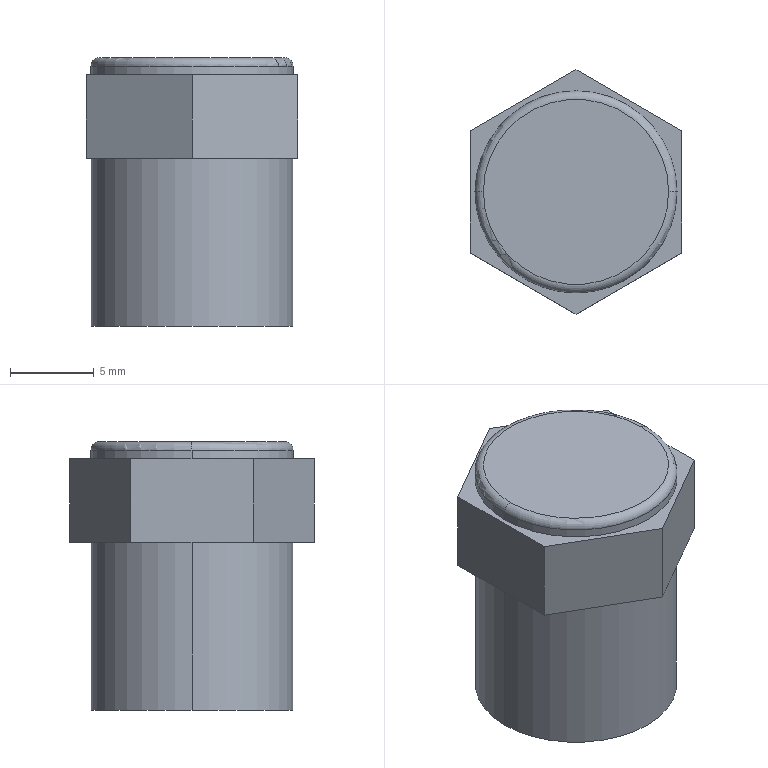Part | SolidWorks | features ICE 2, Extrusion 1, Fillet 1 | 1 solid | 16 faces | box 12.619 x 14.572 x 16 mm | volume 1932 mm3 | plane 10 | cylinder 4 | torus 2 | commonest cylinder face diameters 12 x2 12.036 x2
STEP:
#1=CARTESIAN_POINT('',(-6.018,0.,15.5));
#2=VERTEX_POINT('',#1);
#3=CARTESIAN_POINT('',(6.018,0.,15.5));
#4=VERTEX_POINT('',#3);
#5=CARTESIAN_POINT('',(0.,0.,15.5));
#6=DIRECTION('',(0.,0.,-1.));
#7=DIRECTION('',(1.,0.,0.));
#8=AXIS2_PLACEMENT_3D('',#5,#6,#7);
#9=CIRCLE('',#8,6.018);
#10=EDGE_CURVE('',#2,#4,#9,.T.);
#11=ORIENTED_EDGE('',*,*,#10,.F.);
#12=CARTESIAN_POINT('',(-5.518,0.,16.));
#13=VERTEX_POINT('',#12);
#14=CARTESIAN_POINT('',(-5.518,0.,15.5));
#15=DIRECTION('',(0.,1.,0.));
#16=DIRECTION('',(-1.,0.,0.));
#17=AXIS2_PLACEMENT_3D('',#14,#15,#16);
#18=CIRCLE('',#17,0.5);
#19=EDGE_CURVE('',#2,#13,#18,.T.);
#20=ORIENTED_EDGE('',*,*,#19,.T.);
#21=CARTESIAN_POINT('',(5.518,0.,16.));
#22=VERTEX_POINT('',#21);
#23=CARTESIAN_POINT('',(0.,0.,16.));
#24=DIRECTION('',(0.,0.,1.));
#25=DIRECTION('',(1.,0.,0.));
#26=AXIS2_PLACEMENT_3D('',#23,#24,#25);
#27=CIRCLE('',#26,5.518);
#28=EDGE_CURVE('',#22,#13,#27,.T.);
#29=ORIENTED_EDGE('',*,*,#28,.F.);
#30=CARTESIAN_POINT('',(5.518,0.,15.5));
#31=DIRECTION('',(0.,-1.,0.));
#32=DIRECTION('',(0.,0.,-1.));
#33=AXIS2_PLACEMENT_3D('',#30,#31,#32);
#34=CIRCLE('',#33,0.5);
#35=EDGE_CURVE('',#4,#22,#34,.T.);
#36=ORIENTED_EDGE('',*,*,#35,.F.);
#37=EDGE_LOOP('',(#11,#20,#29,#36));
#38=FACE_OUTER_BOUND('',#37,.T.);
#39=CARTESIAN_POINT('',(0.,0.,15.5));
#40=DIRECTION('',(0.,0.,1.));
#41=DIRECTION('',(1.,0.,0.));
#42=AXIS2_PLACEMENT_3D('',#39,#40,#41);
#43=TOROIDAL_SURFACE('',#42,5.518,0.5);
#44=ADVANCED_FACE('',(#38),#43,.T.);
#45=ORIENTED_EDGE('',*,*,#10,.T.);
#46=CARTESIAN_POINT('',(6.018,0.,15.));
#47=VERTEX_POINT('',#46);
#48=CARTESIAN_POINT('',(6.018,0.,16.));
#49=DIRECTION('',(0.,0.,-1.));
#50=VECTOR('',#49,1000.);
#51=LINE('',#48,#50);
#52=EDGE_CURVE('',#4,#47,#51,.T.);
#53=ORIENTED_EDGE('',*,*,#52,.T.);
#54=CARTESIAN_POINT('',(-6.018,0.,15.));
#55=VERTEX_POINT('',#54);
#56=CARTESIAN_POINT('',(0.,0.,15.));
#57=DIRECTION('',(0.,0.,1.));
#58=DIRECTION('',(1.,0.,0.));
#59=AXIS2_PLACEMENT_3D('',#56,#57,#58);
#60=CIRCLE('',#59,6.018);
#61=EDGE_CURVE('',#47,#55,#60,.T.);
#62=ORIENTED_EDGE('',*,*,#61,.T.);
#63=CARTESIAN_POINT('',(-6.018,0.,16.));
#64=DIRECTION('',(0.,0.,-1.));
#65=VECTOR('',#64,1000.);
#66=LINE('',#63,#65);
#67=EDGE_CURVE('',#2,#55,#66,.T.);
#68=ORIENTED_EDGE('',*,*,#67,.F.);
#69=EDGE_LOOP('',(#45,#53,#62,#68));
#70=FACE_OUTER_BOUND('',#69,.T.);
#71=CARTESIAN_POINT('',(0.,0.,16.));
#72=DIRECTION('',(0.,0.,-1.));
#73=DIRECTION('',(-1.,0.,0.));
#74=AXIS2_PLACEMENT_3D('',#71,#72,#73);
#75=CYLINDRICAL_SURFACE('',#74,6.018);
#76=ADVANCED_FACE('',(#70),#75,.T.);
#77=CARTESIAN_POINT('',(6.,0.,10.));
#78=VERTEX_POINT('',#77);
#79=CARTESIAN_POINT('',(-6.,0.,10.));
#80=VERTEX_POINT('',#79);
#81=CARTESIAN_POINT('',(0.,0.,10.));
#82=DIRECTION('',(0.,0.,1.));
#83=DIRECTION('',(1.,0.,0.));
#84=AXIS2_PLACEMENT_3D('',#81,#82,#83);
#85=CIRCLE('',#84,6.);
#86=EDGE_CURVE('',#78,#80,#85,.T.);
#87=ORIENTED_EDGE('',*,*,#86,.F.);
#88=CARTESIAN_POINT('',(6.,0.,0.));
#89=VERTEX_POINT('',#88);
#90=CARTESIAN_POINT('',(6.,0.,10.));
#91=DIRECTION('',(0.,0.,-1.));
#92=VECTOR('',#91,1000.);
#93=LINE('',#90,#92);
#94=EDGE_CURVE('',#78,#89,#93,.T.);
#95=ORIENTED_EDGE('',*,*,#94,.T.);
#96=CARTESIAN_POINT('',(-6.,0.,0.));
#97=VERTEX_POINT('',#96);
#98=CARTESIAN_POINT('',(0.,0.,0.));
#99=DIRECTION('',(0.,0.,1.));
#100=DIRECTION('',(1.,0.,0.));
#101=AXIS2_PLACEMENT_3D('',#98,#99,#100);
#102=CIRCLE('',#101,6.);
#103=EDGE_CURVE('',#89,#97,#102,.T.);
#104=ORIENTED_EDGE('',*,*,#103,.T.);
#105=CARTESIAN_POINT('',(-6.,0.,10.));
#106=DIRECTION('',(0.,0.,-1.));
#107=VECTOR('',#106,1000.);
#108=LINE('',#105,#107);
#109=EDGE_CURVE('',#80,#97,#108,.T.);
#110=ORIENTED_EDGE('',*,*,#109,.F.);
#111=EDGE_LOOP('',(#87,#95,#104,#110));
#112=FACE_OUTER_BOUND('',#111,.T.);
#113=CARTESIAN_POINT('',(0.,0.,10.));
#114=DIRECTION('',(0.,0.,-1.));
#115=DIRECTION('',(-1.,0.,0.));
#116=AXIS2_PLACEMENT_3D('',#113,#114,#115);
#117=CYLINDRICAL_SURFACE('',#116,6.);
#118=ADVANCED_FACE('',(#112),#117,.T.);
#119=ORIENTED_EDGE('',*,*,#94,.F.);
#120=CARTESIAN_POINT('',(0.,0.,10.));
#121=DIRECTION('',(0.,0.,1.));
#122=DIRECTION('',(1.,0.,0.));
#123=AXIS2_PLACEMENT_3D('',#120,#121,#122);
#124=CIRCLE('',#123,6.);
#125=EDGE_CURVE('',#80,#78,#124,.T.);
#126=ORIENTED_EDGE('',*,*,#125,.F.);
#127=ORIENTED_EDGE('',*,*,#109,.T.);
#128=CARTESIAN_POINT('',(0.,0.,0.));
#129=DIRECTION('',(0.,0.,1.));
#130=DIRECTION('',(1.,0.,0.));
#131=AXIS2_PLACEMENT_3D('',#128,#129,#130);
#132=CIRCLE('',#131,6.);
#133=EDGE_CURVE('',#97,#89,#132,.T.);
#134=ORIENTED_EDGE('',*,*,#133,.T.);
#135=EDGE_LOOP('',(#119,#126,#127,#134));
#136=FACE_OUTER_BOUND('',#135,.T.);
#137=CARTESIAN_POINT('',(0.,0.,10.));
#138=DIRECTION('',(0.,0.,-1.));
#139=DIRECTION('',(-1.,0.,0.));
#140=AXIS2_PLACEMENT_3D('',#137,#138,#139);
#141=CYLINDRICAL_SURFACE('',#140,6.);
#142=ADVANCED_FACE('',(#136),#141,.T.);
#143=ORIENTED_EDGE('',*,*,#133,.F.);
#144=ORIENTED_EDGE('',*,*,#103,.F.);
#145=EDGE_LOOP('',(#143,#144));
#146=FACE_OUTER_BOUND('',#145,.T.);
#147=CARTESIAN_POINT('',(0.,0.,0.));
#148=DIRECTION('',(0.,0.,1.));
#149=DIRECTION('',(1.,0.,0.));
#150=AXIS2_PLACEMENT_3D('',#147,#148,#149);
#151=PLANE('',#150);
#152=ADVANCED_FACE('',(#146),#151,.F.);
#153=CARTESIAN_POINT('',(6.31,3.643,10.));
#154=VERTEX_POINT('',#153);
#155=CARTESIAN_POINT('',(0.,7.286,10.));
#156=VERTEX_POINT('',#155);
#157=CARTESIAN_POINT('',(6.31,3.643,10.));
#158=DIRECTION('',(-0.866,0.5,0.));
#159=VECTOR('',#158,1000.);
#160=LINE('',#157,#159);
#161=EDGE_CURVE('',#154,#156,#160,.T.);
#162=ORIENTED_EDGE('',*,*,#161,.T.);
#163=CARTESIAN_POINT('',(0.,7.286,15.));
#164=VERTEX_POINT('',#163);
#165=CARTESIAN_POINT('',(0.,7.286,15.));
#166=DIRECTION('',(0.,0.,-1.));
#167=VECTOR('',#166,1000.);
#168=LINE('',#165,#167);
#169=EDGE_CURVE('',#164,#156,#168,.T.);
#170=ORIENTED_EDGE('',*,*,#169,.F.);
#171=CARTESIAN_POINT('',(6.31,3.643,15.));
#172=VERTEX_POINT('',#171);
#173=CARTESIAN_POINT('',(6.31,3.643,15.));
#174=DIRECTION('',(-0.866,0.5,0.));
#175=VECTOR('',#174,1000.);
#176=LINE('',#173,#175);
#177=EDGE_CURVE('',#172,#164,#176,.T.);
#178=ORIENTED_EDGE('',*,*,#177,.F.);
#179=CARTESIAN_POINT('',(6.31,3.643,15.));
#180=DIRECTION('',(0.,0.,-1.));
#181=VECTOR('',#180,1000.);
#182=LINE('',#179,#181);
#183=EDGE_CURVE('',#172,#154,#182,.T.);
#184=ORIENTED_EDGE('',*,*,#183,.T.);
#185=EDGE_LOOP('',(#162,#170,#178,#184));
#186=FACE_OUTER_BOUND('',#185,.T.);
#187=CARTESIAN_POINT('',(6.31,3.643,15.));
#188=DIRECTION('',(-0.5,-0.866,0.));
#189=DIRECTION('',(0.866,-0.5,0.));
#190=AXIS2_PLACEMENT_3D('',#187,#188,#189);
#191=PLANE('',#190);
#192=ADVANCED_FACE('',(#186),#191,.F.);
#193=CARTESIAN_POINT('',(-6.31,3.643,10.));
#194=VERTEX_POINT('',#193);
#195=CARTESIAN_POINT('',(0.,7.286,10.));
#196=DIRECTION('',(-0.866,-0.5,0.));
#197=VECTOR('',#196,1000.);
#198=LINE('',#195,#197);
#199=EDGE_CURVE('',#156,#194,#198,.T.);
#200=ORIENTED_EDGE('',*,*,#199,.T.);
#201=CARTESIAN_POINT('',(-6.31,3.643,15.));
#202=VERTEX_POINT('',#201);
#203=CARTESIAN_POINT('',(-6.31,3.643,15.));
#204=DIRECTION('',(0.,0.,-1.));
#205=VECTOR('',#204,1000.);
#206=LINE('',#203,#205);
#207=EDGE_CURVE('',#202,#194,#206,.T.);
#208=ORIENTED_EDGE('',*,*,#207,.F.);
#209=CARTESIAN_POINT('',(0.,7.286,15.));
#210=DIRECTION('',(-0.866,-0.5,0.));
#211=VECTOR('',#210,1000.);
#212=LINE('',#209,#211);
#213=EDGE_CURVE('',#164,#202,#212,.T.);
#214=ORIENTED_EDGE('',*,*,#213,.F.);
#215=ORIENTED_EDGE('',*,*,#169,.T.);
#216=EDGE_LOOP('',(#200,#208,#214,#215));
#217=FACE_OUTER_BOUND('',#216,.T.);
#218=CARTESIAN_POINT('',(0.,7.286,15.));
#219=DIRECTION('',(0.5,-0.866,0.));
#220=DIRECTION('',(0.866,0.5,0.));
#221=AXIS2_PLACEMENT_3D('',#218,#219,#220);
#222=PLANE('',#221);
#223=ADVANCED_FACE('',(#217),#222,.F.);
#224=CARTESIAN_POINT('',(-6.31,-3.643,10.));
#225=VERTEX_POINT('',#224);
#226=CARTESIAN_POINT('',(-6.31,3.643,10.));
#227=DIRECTION('',(0.,-1.,0.));
#228=VECTOR('',#227,1000.);
#229=LINE('',#226,#228);
#230=EDGE_CURVE('',#194,#225,#229,.T.);
#231=ORIENTED_EDGE('',*,*,#230,.T.);
#232=CARTESIAN_POINT('',(-6.31,-3.643,15.));
#233=VERTEX_POINT('',#232);
#234=CARTESIAN_POINT('',(-6.31,-3.643,15.));
#235=DIRECTION('',(0.,0.,-1.));
#236=VECTOR('',#235,1000.);
#237=LINE('',#234,#236);
#238=EDGE_CURVE('',#233,#225,#237,.T.);
#239=ORIENTED_EDGE('',*,*,#238,.F.);
#240=CARTESIAN_POINT('',(-6.31,3.643,15.));
#241=DIRECTION('',(0.,-1.,0.));
#242=VECTOR('',#241,1000.);
#243=LINE('',#240,#242);
#244=EDGE_CURVE('',#202,#233,#243,.T.);
#245=ORIENTED_EDGE('',*,*,#244,.F.);
#246=ORIENTED_EDGE('',*,*,#207,.T.);
#247=EDGE_LOOP('',(#231,#239,#245,#246));
#248=FACE_OUTER_BOUND('',#247,.T.);
#249=CARTESIAN_POINT('',(-6.31,3.643,15.));
#250=DIRECTION('',(1.,0.,0.));
#251=DIRECTION('',(0.,1.,0.));
#252=AXIS2_PLACEMENT_3D('',#249,#250,#251);
#253=PLANE('',#252);
#254=ADVANCED_FACE('',(#248),#253,.F.);
#255=CARTESIAN_POINT('',(0.,-7.286,10.));
#256=VERTEX_POINT('',#255);
#257=CARTESIAN_POINT('',(-6.31,-3.643,10.));
#258=DIRECTION('',(0.866,-0.5,0.));
#259=VECTOR('',#258,1000.);
#260=LINE('',#257,#259);
#261=EDGE_CURVE('',#225,#256,#260,.T.);
#262=ORIENTED_EDGE('',*,*,#261,.T.);
#263=CARTESIAN_POINT('',(0.,-7.286,15.));
#264=VERTEX_POINT('',#263);
#265=CARTESIAN_POINT('',(0.,-7.286,15.));
#266=DIRECTION('',(0.,0.,-1.));
#267=VECTOR('',#266,1000.);
#268=LINE('',#265,#267);
#269=EDGE_CURVE('',#264,#256,#268,.T.);
#270=ORIENTED_EDGE('',*,*,#269,.F.);
#271=CARTESIAN_POINT('',(-6.31,-3.643,15.));
#272=DIRECTION('',(0.866,-0.5,0.));
#273=VECTOR('',#272,1000.);
#274=LINE('',#271,#273);
#275=EDGE_CURVE('',#233,#264,#274,.T.);
#276=ORIENTED_EDGE('',*,*,#275,.F.);
#277=ORIENTED_EDGE('',*,*,#238,.T.);
#278=EDGE_LOOP('',(#262,#270,#276,#277));
#279=FACE_OUTER_BOUND('',#278,.T.);
#280=CARTESIAN_POINT('',(-6.31,-3.643,15.));
#281=DIRECTION('',(0.5,0.866,0.));
#282=DIRECTION('',(-0.866,0.5,0.));
#283=AXIS2_PLACEMENT_3D('',#280,#281,#282);
#284=PLANE('',#283);
#285=ADVANCED_FACE('',(#279),#284,.F.);
#286=CARTESIAN_POINT('',(6.31,-3.643,10.));
#287=VERTEX_POINT('',#286);
#288=CARTESIAN_POINT('',(0.,-7.286,10.));
#289=DIRECTION('',(0.866,0.5,0.));
#290=VECTOR('',#289,1000.);
#291=LINE('',#288,#290);
#292=EDGE_CURVE('',#256,#287,#291,.T.);
#293=ORIENTED_EDGE('',*,*,#292,.T.);
#294=CARTESIAN_POINT('',(6.31,-3.643,15.));
#295=VERTEX_POINT('',#294);
#296=CARTESIAN_POINT('',(6.31,-3.643,15.));
#297=DIRECTION('',(0.,0.,-1.));
#298=VECTOR('',#297,1000.);
#299=LINE('',#296,#298);
#300=EDGE_CURVE('',#295,#287,#299,.T.);
#301=ORIENTED_EDGE('',*,*,#300,.F.);
#302=CARTESIAN_POINT('',(0.,-7.286,15.));
#303=DIRECTION('',(0.866,0.5,0.));
#304=VECTOR('',#303,1000.);
#305=LINE('',#302,#304);
#306=EDGE_CURVE('',#264,#295,#305,.T.);
#307=ORIENTED_EDGE('',*,*,#306,.F.);
#308=ORIENTED_EDGE('',*,*,#269,.T.);
#309=EDGE_LOOP('',(#293,#301,#307,#308));
#310=FACE_OUTER_BOUND('',#309,.T.);
#311=CARTESIAN_POINT('',(0.,-7.286,15.));
#312=DIRECTION('',(-0.5,0.866,0.));
#313=DIRECTION('',(-0.866,-0.5,0.));
#314=AXIS2_PLACEMENT_3D('',#311,#312,#313);
#315=PLANE('',#314);
#316=ADVANCED_FACE('',(#310),#315,.F.);
#317=CARTESIAN_POINT('',(6.31,-3.643,10.));
#318=DIRECTION('',(0.,1.,0.));
#319=VECTOR('',#318,1000.);
#320=LINE('',#317,#319);
#321=EDGE_CURVE('',#287,#154,#320,.T.);
#322=ORIENTED_EDGE('',*,*,#321,.T.);
#323=ORIENTED_EDGE('',*,*,#183,.F.);
#324=CARTESIAN_POINT('',(6.31,-3.643,15.));
#325=DIRECTION('',(0.,1.,0.));
#326=VECTOR('',#325,1000.);
#327=LINE('',#324,#326);
#328=EDGE_CURVE('',#295,#172,#327,.T.);
#329=ORIENTED_EDGE('',*,*,#328,.F.);
#330=ORIENTED_EDGE('',*,*,#300,.T.);
#331=EDGE_LOOP('',(#322,#323,#329,#330));
#332=FACE_OUTER_BOUND('',#331,.T.);
#333=CARTESIAN_POINT('',(6.31,-3.643,15.));
#334=DIRECTION('',(-1.,0.,0.));
#335=DIRECTION('',(0.,-1.,0.));
#336=AXIS2_PLACEMENT_3D('',#333,#334,#335);
#337=PLANE('',#336);
#338=ADVANCED_FACE('',(#332),#337,.F.);
#339=CARTESIAN_POINT('',(0.,0.,15.));
#340=DIRECTION('',(0.,0.,1.));
#341=DIRECTION('',(1.,0.,0.));
#342=AXIS2_PLACEMENT_3D('',#339,#340,#341);
#343=CIRCLE('',#342,6.018);
#344=EDGE_CURVE('',#55,#47,#343,.T.);
#345=ORIENTED_EDGE('',*,*,#344,.F.);
#346=ORIENTED_EDGE('',*,*,#61,.F.);
#347=EDGE_LOOP('',(#345,#346));
#348=FACE_BOUND('',#347,.T.);
#349=ORIENTED_EDGE('',*,*,#177,.T.);
#350=ORIENTED_EDGE('',*,*,#213,.T.);
#351=ORIENTED_EDGE('',*,*,#244,.T.);
#352=ORIENTED_EDGE('',*,*,#275,.T.);
#353=ORIENTED_EDGE('',*,*,#306,.T.);
#354=ORIENTED_EDGE('',*,*,#328,.T.);
#355=EDGE_LOOP('',(#349,#350,#351,#352,#353,#354));
#356=FACE_OUTER_BOUND('',#355,.T.);
#357=CARTESIAN_POINT('',(0.,0.,15.));
#358=DIRECTION('',(0.,0.,1.));
#359=DIRECTION('',(1.,0.,0.));
#360=AXIS2_PLACEMENT_3D('',#357,#358,#359);
#361=PLANE('',#360);
#362=ADVANCED_FACE('',(#348,#356),#361,.T.);
#363=ORIENTED_EDGE('',*,*,#125,.T.);
#364=ORIENTED_EDGE('',*,*,#86,.T.);
#365=EDGE_LOOP('',(#363,#364));
#366=FACE_BOUND('',#365,.T.);
#367=ORIENTED_EDGE('',*,*,#161,.F.);
#368=ORIENTED_EDGE('',*,*,#321,.F.);
#369=ORIENTED_EDGE('',*,*,#292,.F.);
#370=ORIENTED_EDGE('',*,*,#261,.F.);
#371=ORIENTED_EDGE('',*,*,#230,.F.);
#372=ORIENTED_EDGE('',*,*,#199,.F.);
#373=EDGE_LOOP('',(#367,#368,#369,#370,#371,#372));
#374=FACE_OUTER_BOUND('',#373,.T.);
#375=CARTESIAN_POINT('',(0.,0.,10.));
#376=DIRECTION('',(0.,0.,1.));
#377=DIRECTION('',(1.,0.,0.));
#378=AXIS2_PLACEMENT_3D('',#375,#376,#377);
#379=PLANE('',#378);
#380=ADVANCED_FACE('',(#366,#374),#379,.F.);
#381=ORIENTED_EDGE('',*,*,#52,.F.);
#382=CARTESIAN_POINT('',(0.,0.,15.5));
#383=DIRECTION('',(0.,0.,-1.));
#384=DIRECTION('',(1.,0.,0.));
#385=AXIS2_PLACEMENT_3D('',#382,#383,#384);
#386=CIRCLE('',#385,6.018);
#387=EDGE_CURVE('',#4,#2,#386,.T.);
#388=ORIENTED_EDGE('',*,*,#387,.T.);
#389=ORIENTED_EDGE('',*,*,#67,.T.);
#390=ORIENTED_EDGE('',*,*,#344,.T.);
#391=EDGE_LOOP('',(#381,#388,#389,#390));
#392=FACE_OUTER_BOUND('',#391,.T.);
#393=CARTESIAN_POINT('',(0.,0.,16.));
#394=DIRECTION('',(0.,0.,-1.));
#395=DIRECTION('',(-1.,0.,0.));
#396=AXIS2_PLACEMENT_3D('',#393,#394,#395);
#397=CYLINDRICAL_SURFACE('',#396,6.018);
#398=ADVANCED_FACE('',(#392),#397,.T.);
#399=ORIENTED_EDGE('',*,*,#28,.T.);
#400=CARTESIAN_POINT('',(0.,0.,16.));
#401=DIRECTION('',(0.,0.,1.));
#402=DIRECTION('',(1.,0.,0.));
#403=AXIS2_PLACEMENT_3D('',#400,#401,#402);
#404=CIRCLE('',#403,5.518);
#405=EDGE_CURVE('',#13,#22,#404,.T.);
#406=ORIENTED_EDGE('',*,*,#405,.T.);
#407=EDGE_LOOP('',(#399,#406));
#408=FACE_OUTER_BOUND('',#407,.T.);
#409=CARTESIAN_POINT('',(0.,0.,16.));
#410=DIRECTION('',(0.,0.,1.));
#411=DIRECTION('',(1.,0.,0.));
#412=AXIS2_PLACEMENT_3D('',#409,#410,#411);
#413=PLANE('',#412);
#414=ADVANCED_FACE('',(#408),#413,.T.);
#415=ORIENTED_EDGE('',*,*,#19,.F.);
#416=ORIENTED_EDGE('',*,*,#387,.F.);
#417=ORIENTED_EDGE('',*,*,#35,.T.);
#418=ORIENTED_EDGE('',*,*,#405,.F.);
#419=EDGE_LOOP('',(#415,#416,#417,#418));
#420=FACE_OUTER_BOUND('',#419,.T.);
#421=CARTESIAN_POINT('',(0.,0.,15.5));
#422=DIRECTION('',(0.,0.,1.));
#423=DIRECTION('',(1.,0.,0.));
#424=AXIS2_PLACEMENT_3D('',#421,#422,#423);
#425=TOROIDAL_SURFACE('',#424,5.518,0.5);
#426=ADVANCED_FACE('',(#420),#425,.T.);
#427=CLOSED_SHELL('',(#44,#76,#118,#142,#152,#192,#223,#254,#285,#316,#338,#362,#380,#398,#414,#426));
#428=MANIFOLD_SOLID_BREP('',#427);
#429=CARTESIAN_POINT('',(0.,0.,0.));
#430=DIRECTION('',(0.,0.,1.));
#431=DIRECTION('',(1.,0.,0.));
#432=AXIS2_PLACEMENT_3D('',#429,#430,#431);
#433=(LENGTH_UNIT()NAMED_UNIT(*)SI_UNIT(.MILLI.,.METRE.));
#434=UNCERTAINTY_MEASURE_WITH_UNIT(LENGTH_MEASURE(0.00001),#433,'','');
#435=(NAMED_UNIT(*)PLANE_ANGLE_UNIT()SI_UNIT($,.RADIAN.));
#436=(NAMED_UNIT(*)SI_UNIT($,.STERADIAN.)SOLID_ANGLE_UNIT());
#437=(GEOMETRIC_REPRESENTATION_CONTEXT(3)GLOBAL_UNCERTAINTY_ASSIGNED_CONTEXT((#434))GLOBAL_UNIT_ASSIGNED_CONTEXT((#433,#435,#436))REPRESENTATION_CONTEXT('',''));
#438=ADVANCED_BREP_SHAPE_REPRESENTATION('',(#428,#432),#437);